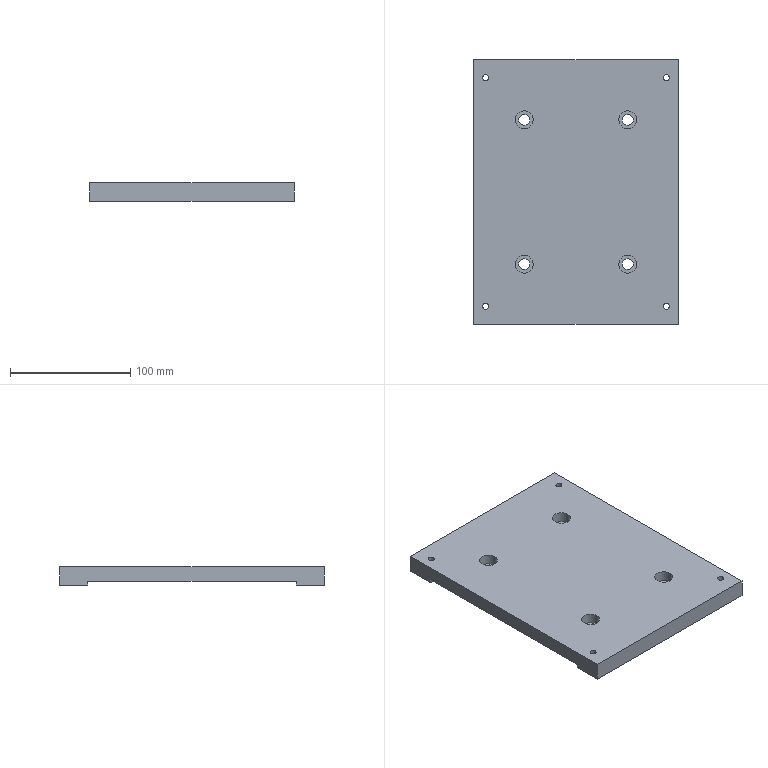Part | STEP file | 44-02-013 Press-fit Fixing Plate | 1 solid | 38 faces | box 170 x 220 x 15 mm | volume 464467 mm3 | cylinder 24 | plane 14 | commonest cylinder face diameters 5 x8 9 x8 15 x8